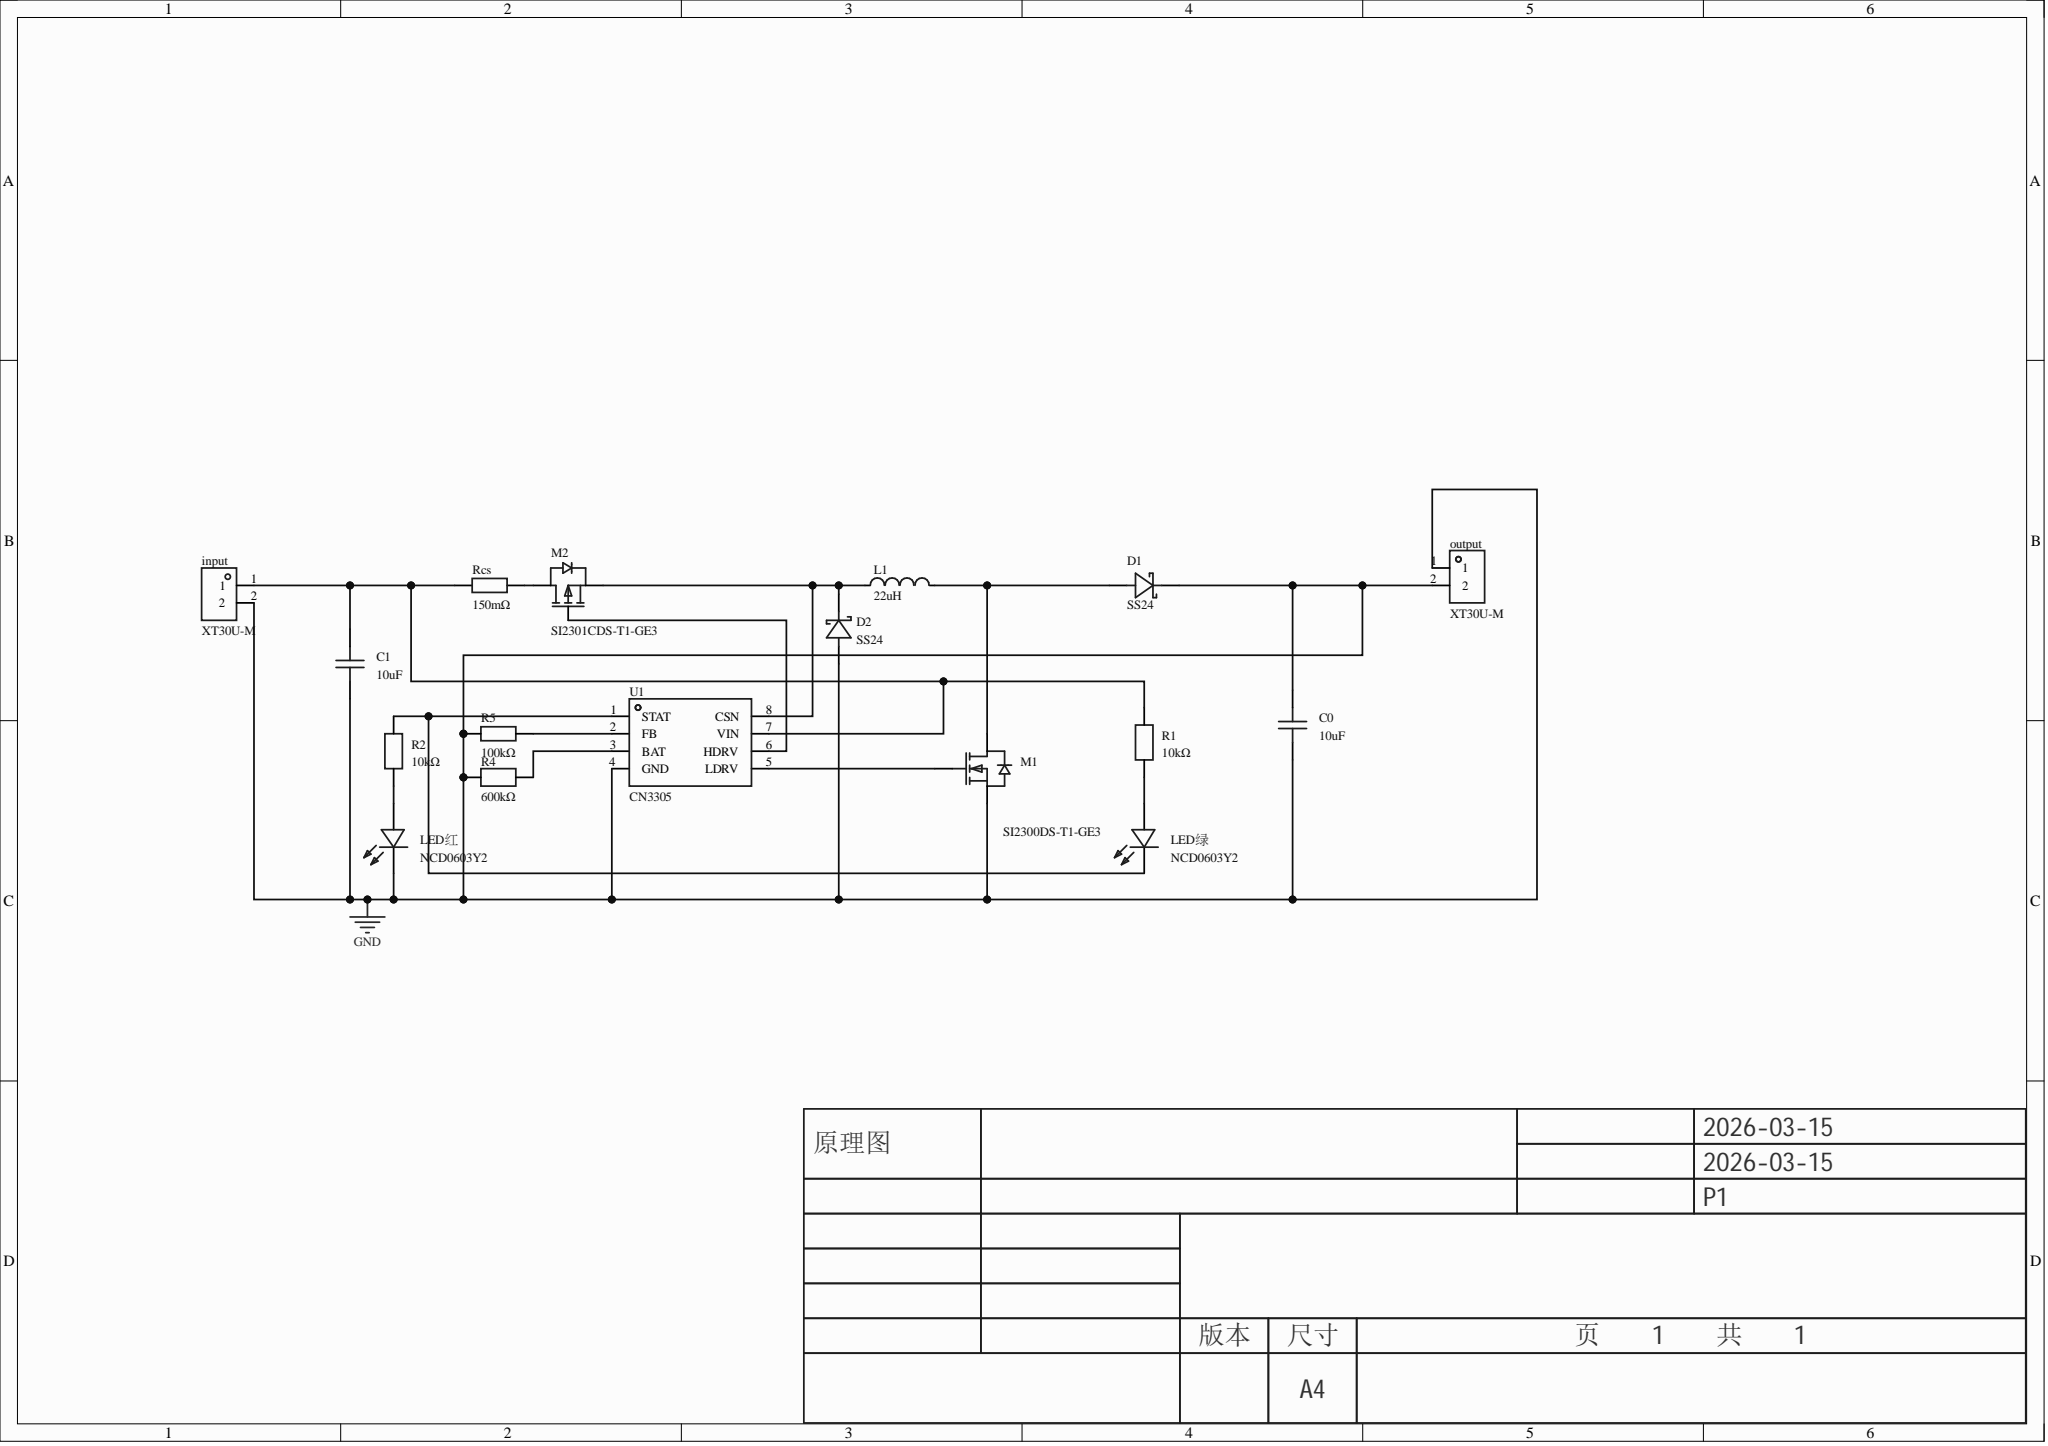Circuit board | Altium Designer | 17 parts | 12 nets
Bill of materials:
Comment,Description,Designator,Footprint,LibRef,Quantity
"10uF","","C0, C1","C0805","CGA0805X5R106K250MT","2"
"SS24","","D1, D2","SMA_L4.3-W2.6-LS5.0-FD","SS24_C7420362","2"
"XT30U-M","","input, output","CONN-TH_XT30U-M","XT30U-M","2"
"22uH","","L1","IND-SMD_L7.0-W6.6_FXL0630","FXL0630-220-M","1"
"NCD0603Y2","","LED红, LED绿","LED0603-RD","NCD0603Y2","2"
"SI2300DS-T1-GE3","","M1","SOT-23-3_L2.9-W1.6-P1.90-LS2.8-BR","SI2300DS-T1-GE3","1"
"SI2301CDS-T1-GE3","","M2","SOT-23-3_L3.0-W1.7-P0.95-LS2.9-BR","SI2301CDS-T1-GE3","1"
"10kΩ","","R1, R2","R0805","FRR0805J103 TS","2"
"600kΩ","","R4","RES-TH_BD3.7-L8.7-P12.8-D0.8","RN60D6003FB14","1"
"100kΩ","","R5","RES-TH_BD2.7-L6.2-P10.20-D0.4","MF1/4W-100K±1%-OT26","1"
"150mΩ","","Rcs","R1206","1206W4F150LT5E","1"
"CN3305","","U1","SOP-8_L4.9-W3.9-P1.27-LS6.0-BL-1","CN3305","1"
Netlist (Protel format):
[
C0
C0805
10uF



]
[
C1
C0805
10uF



]
[
D1
SMA_L4.3-W2.6-LS5.0-FD
SS24



]
[
D2
SMA_L4.3-W2.6-LS5.0-FD
SS24



]
[
input
CONN-TH_XT30U-M
XT30U-M



]
[
L1
IND-SMD_L7.0-W6.6_FXL0630
22uH



]
[
LED红
LED0603-RD
NCD0603Y2



]
[
LED绿
LED0603-RD
NCD0603Y2



]
[
M1
SOT-23-3_L2.9-W1.6-P1.90-LS2.8-BR
SI2300DS-T1-GE3



]
[
M2
SOT-23-3_L3.0-W1.7-P0.95-LS2.9-BR
SI2301CDS-T1-GE3



]
[
output
CONN-TH_XT30U-M
XT30U-M



]
[
R1
R0805
10kΩ



]
[
R2
R0805
10kΩ



]
[
R4
RES-TH_BD3.7-L8.7-P12.8-D0.8
600kΩ



]
[
R5
RES-TH_BD2.7-L6.2-P10.20-D0.4
100kΩ



]
[
Rcs
R1206
150mΩ



]
[
U1
SOP-8_L4.9-W3.9-P1.27-LS6.0-BL-1
CN3305



]
(
NetR5_2
R5-2
U1-2
)
(
NetR4_2
R4-2
U1-3
)
(
NetM2_3
M2-3
Rcs-2
)
(
NetM2_1
M2-1
U1-6
)
(
NetM1_1
M1-1
U1-5
)
(
NetLED绿_2
LED绿-2
R1-1
)
(
NetLED绿_1
LED绿-1
R2-2
U1-1
)
(
NetLED红_2
LED红-2
R2-1
)
(
NetD2_2
D2-2
L1-1
M2-2
U1-8
)
(
NetD1_1
D1-1
L1-2
M1-3
)
(
NetC1_2
C1-2
input-1
R1-2
Rcs-1
U1-7
)
(
GND
C0-1
C0-2
C1-1
D1-2
D2-1
input-2
LED红-1
M1-2
output-1
output-2
R4-1
R5-1
U1-4
)